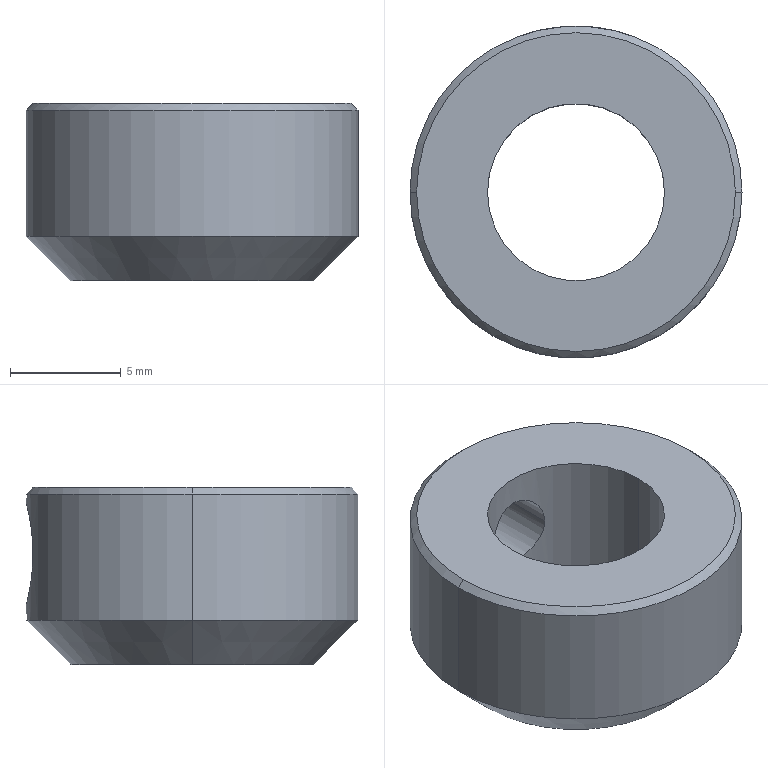Part | NX | 1 solid | 14 faces | box 15 x 15 x 8 mm | volume 892.084 mm3 | cylinder 6 | cone 4 | spline 2 | plane 2 | commonest cylinder face diameters 3.3 x2 8 x2 15 x2